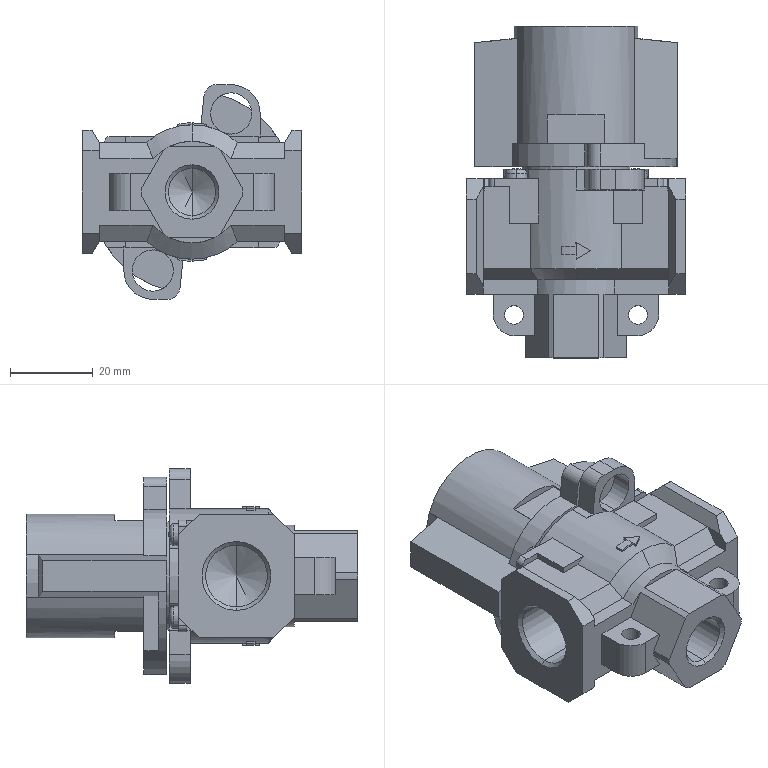Part | STEP file | 11-GYVHS30-03A-30-V10-22111.11 | 1 solid | 249 faces | box 53 x 80.3 x 52 mm | volume 74557 mm3 | plane 152 | cylinder 56 | cone 25 | sphere 8 | torus 8 | commonest cylinder face diameters 10 x6 24.6 x5 3 x4 4.5 x4 6.6 x4 14.95 x4